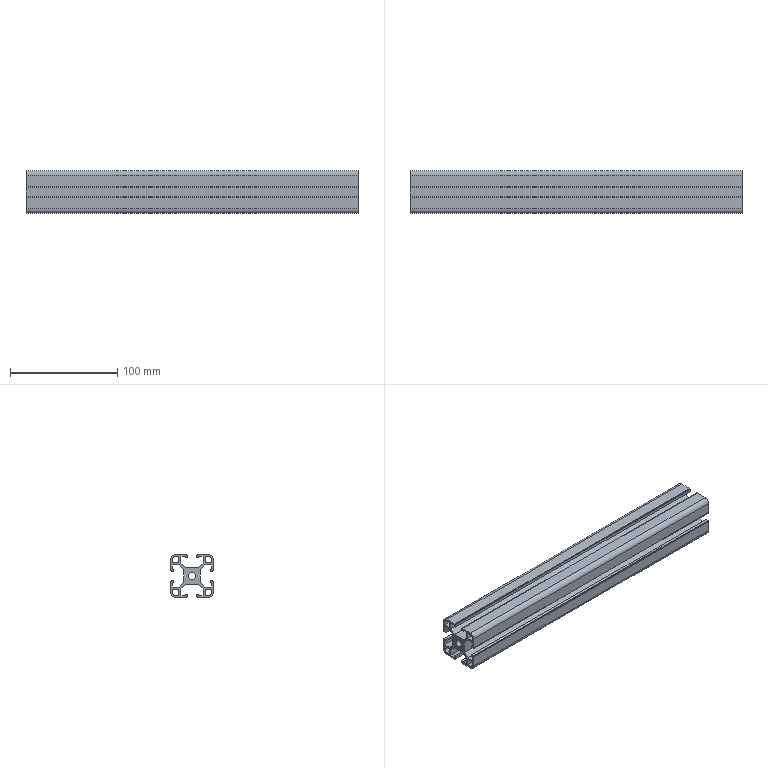Part | SolidWorks | features WeldMemberFeat 1, WeldmentFeature 1 | 1 solid | 104 faces | box 310 x 40 x 40 mm | volume 178729 mm3 | plane 94 | cylinder 10 | commonest cylinder face diameters 5 x4 9 x4 6.8 x2